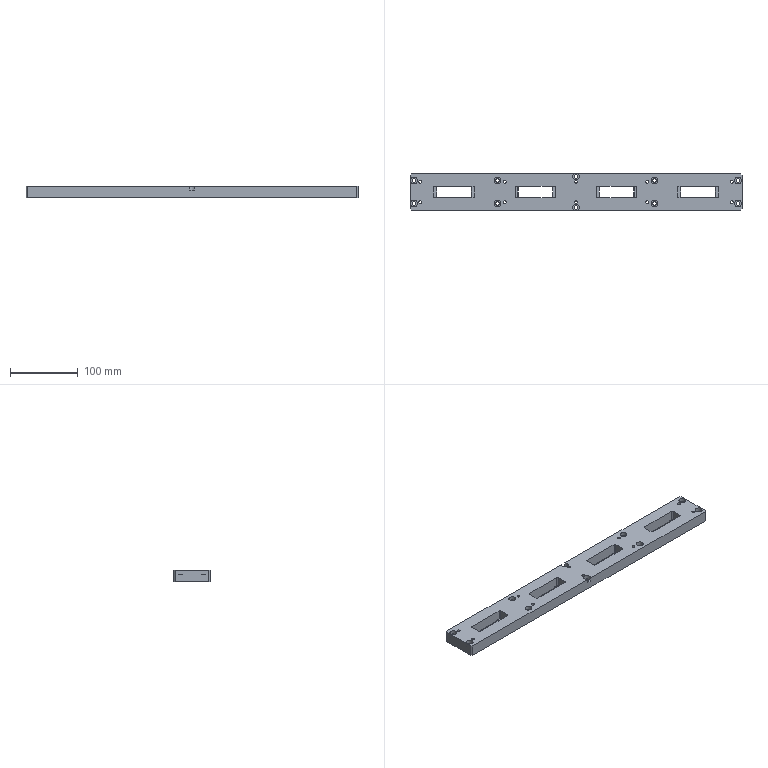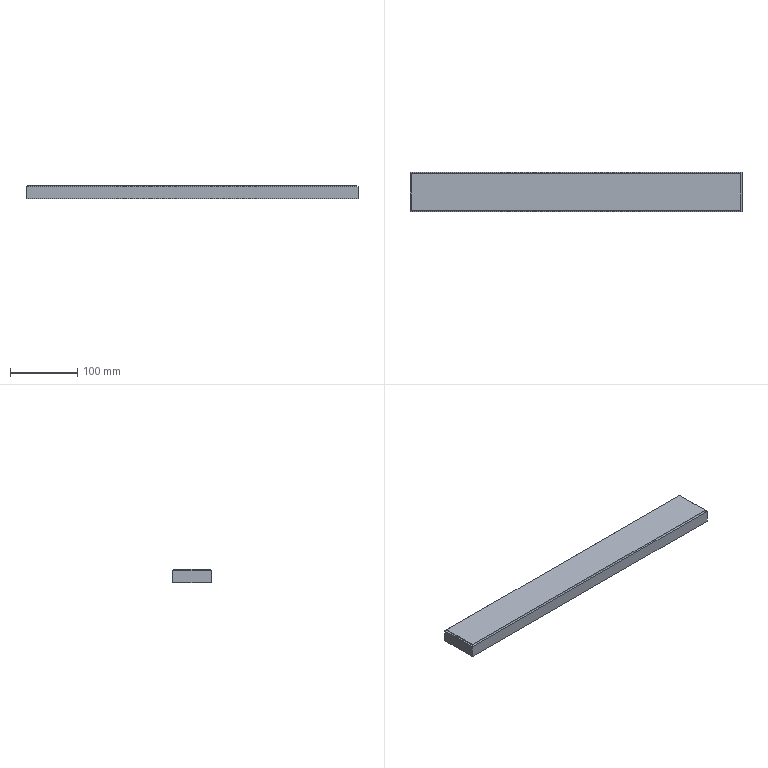CAM job | NX | 3-axis milling, drilling | part box 490 x 54 x 17 mm | stock box 494 x 58 x 20 mm
Tools:
number,name,description,diameter,corner_radius,flute_length,length,flutes
19,D80,Milling Tool-5 Parameters,80.0,0.0,50.0,75.0,2
15,D10,Milling Tool-5 Parameters,10.0,0.0,50.0,75.0,2
1,D6A45,Milling Tool-5 Parameters,6.0,0.0,50.0,75.0,2
4,4..2ZT,Drilling Tool,4.2,0.0,35.0,50.0,2
9,5.5ZT,Drilling Tool,5.5,0.0,35.0,50.0,2
12,D6,Milling Tool-5 Parameters,6.0,0.0,50.0,75.0,2
14,D10JING,Milling Tool-5 Parameters,10.0,0.0,50.0,75.0,2
11,D4,Milling Tool-5 Parameters,4.0,0.0,30.0,30.0,4
5,D4R0.5,Milling Tool-5 Parameters,4.0,0.5,50.0,75.0,2
3,D3,Milling Tool-5 Parameters,3.0,0.0,50.0,75.0,2
Operations:
program,operation,operation_type,tool,method,geometry_group,spindle_rpm,surface_speed,feed_per_tooth,feed_cut,feed_plunge,cut_length_mm,path_length_mm,cut_time_min,machine_time_min
1,FLOOR_WALL,VolumeBased25DMillingOperation,D80,METHOD,A,6500.0,1633.0,0.1154,1500.0,100.0,586.0,640.0,0.3907,0.3961
1,DRILLING,Operation,D6A45,METHOD,A,5000.0,94.0,0.035,350.0,0.0,96.0,1014.825,0.2743,0.3662
1,DRILLING_COPY_COPY,Operation,4..2ZT,METHOD,A,2000.0,26.0,0.075,300.0,0.0,227.618,1153.142,0.7587,0.8513
1,DRILLING_COPY_COPY_COPY,Operation,5.5ZT,METHOD,A,2000.0,34.0,0.075,300.0,0.0,221.524,1191.134,0.7384,0.8354
1,ZLEVEL_PROFILE,ZLevelMilling,D10,METHOD,A,8500.0,267.0,0.1765,3000.0,1000.0,20484.124,21253.8,7.014,7.091
1,ZLEVEL_PROFILE_1,ZLevelMilling,D10JING,METHOD,A,8500.0,267.0,0.0882,1500.0,1000.0,1547.189,2872.389,1.039,1.172
1,ZLEVEL_PROFILE_1_COPY,ZLevelMilling,D10JING,METHOD,A,8500.0,267.0,0.0882,1500.0,1000.0,920.241,2095.269,0.6263,0.7438
1,HOLE_MILLING,CylinderMilling,D6,METHOD,A,8500.0,160.0,0.0853,1450.0,100.0,1488.5,2800.81,1.027,1.158
1,ZLEVEL_PROFILE_COPY,ZLevelMilling,D4,METHOD,A,8500.0,106.0,0.0441,1500.0,1000.0,7106.155,11677.954,5.242,5.699
1,ZLEVEL_PROFILE_2,ZLevelMilling,D4R0.5,METHOD,A,8500.0,106.0,0.1471,2500.0,100.0,1120.848,2238.298,0.4483,0.5601
1,PLANAR_MILL_COPY,PlanarMilling,D6A45,METHOD,A,8500.0,160.0,0.0735,1250.0,100.0,2106.834,4414.097,1.685,1.916
2,FLOOR_WALL_COPY,VolumeBased25DMillingOperation,D80,METHOD,B,6500.0,1633.0,0.1154,1500.0,100.0,1746.0,3054.001,1.164,1.295
2,HOLE_MILLING_1,CylinderMilling,D3,METHOD,B,9500.0,89.0,0.0526,1000.0,100.0,413.362,1032.362,0.4134,0.4753
2,PLANAR_MILL_COPY_COPY,PlanarMilling,D6A45,METHOD,B,9500.0,179.0,0.0658,1250.0,100.0,1417.883,3514.96,1.134,1.344
2,PLANAR_MILL_COPY_COPY_COPY,PlanarMilling,D6A45,METHOD,B,9500.0,179.0,0.0658,1250.0,100.0,539.677,1144.873,0.4317,0.4923
2,刀补,CylinderMilling,D3,METHOD,B,9500.0,89.0,0.0526,1000.0,100.0,84.047,703.048,0.084,0.1459